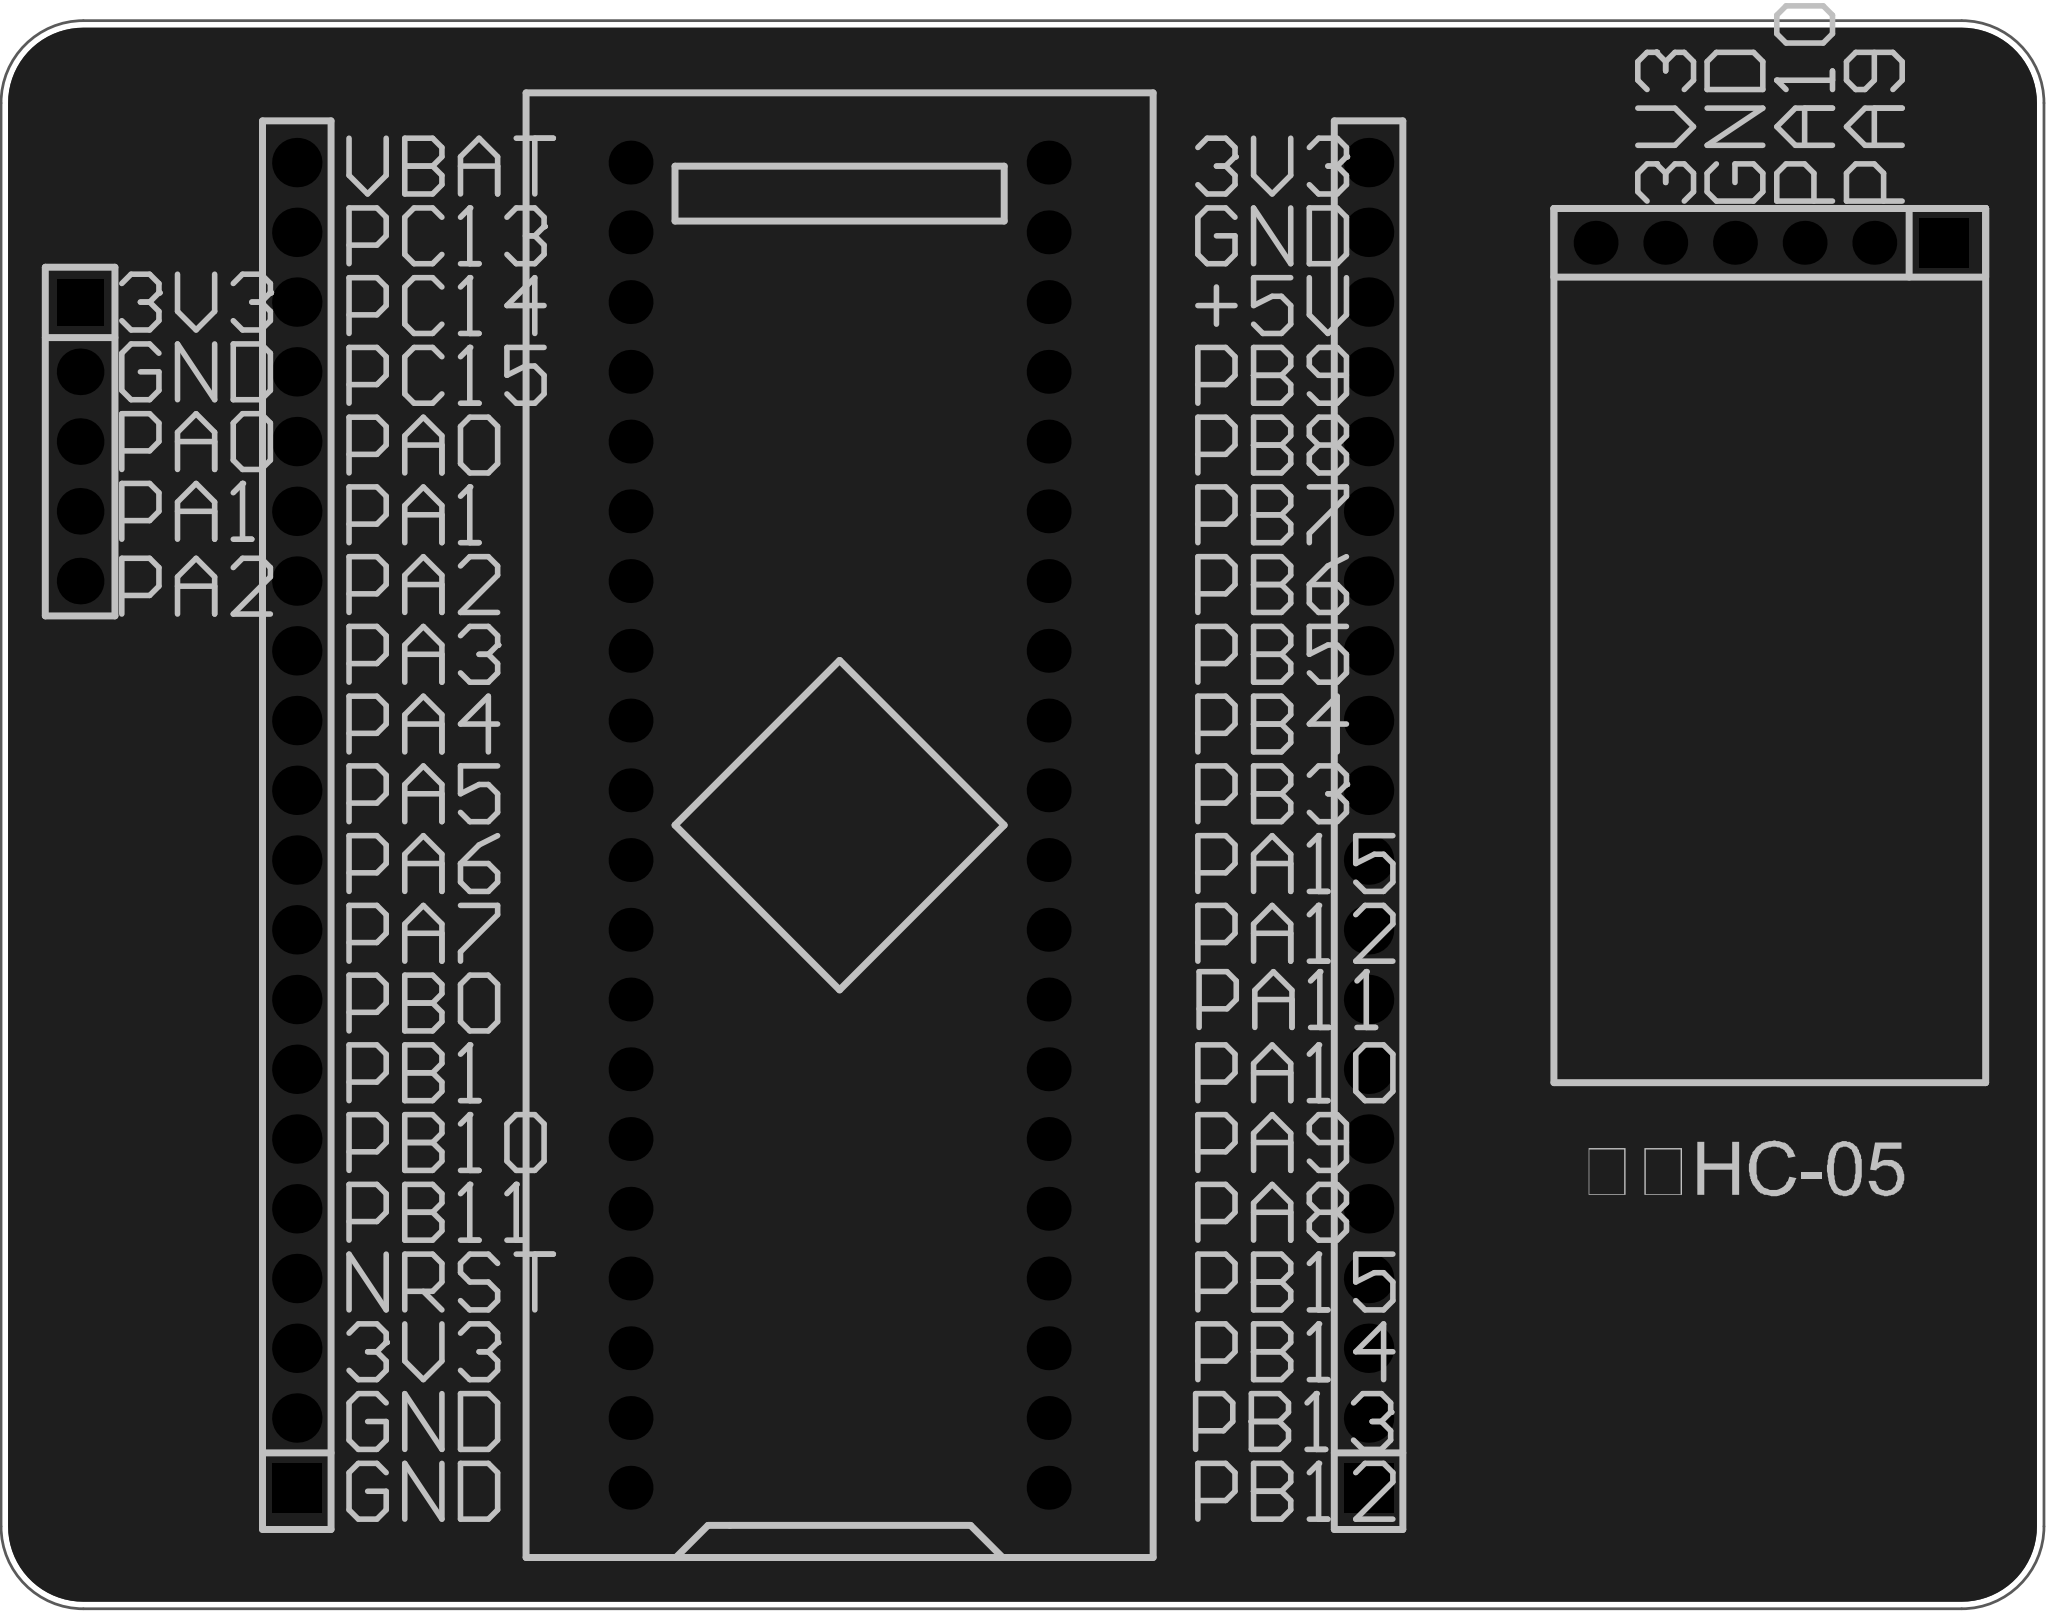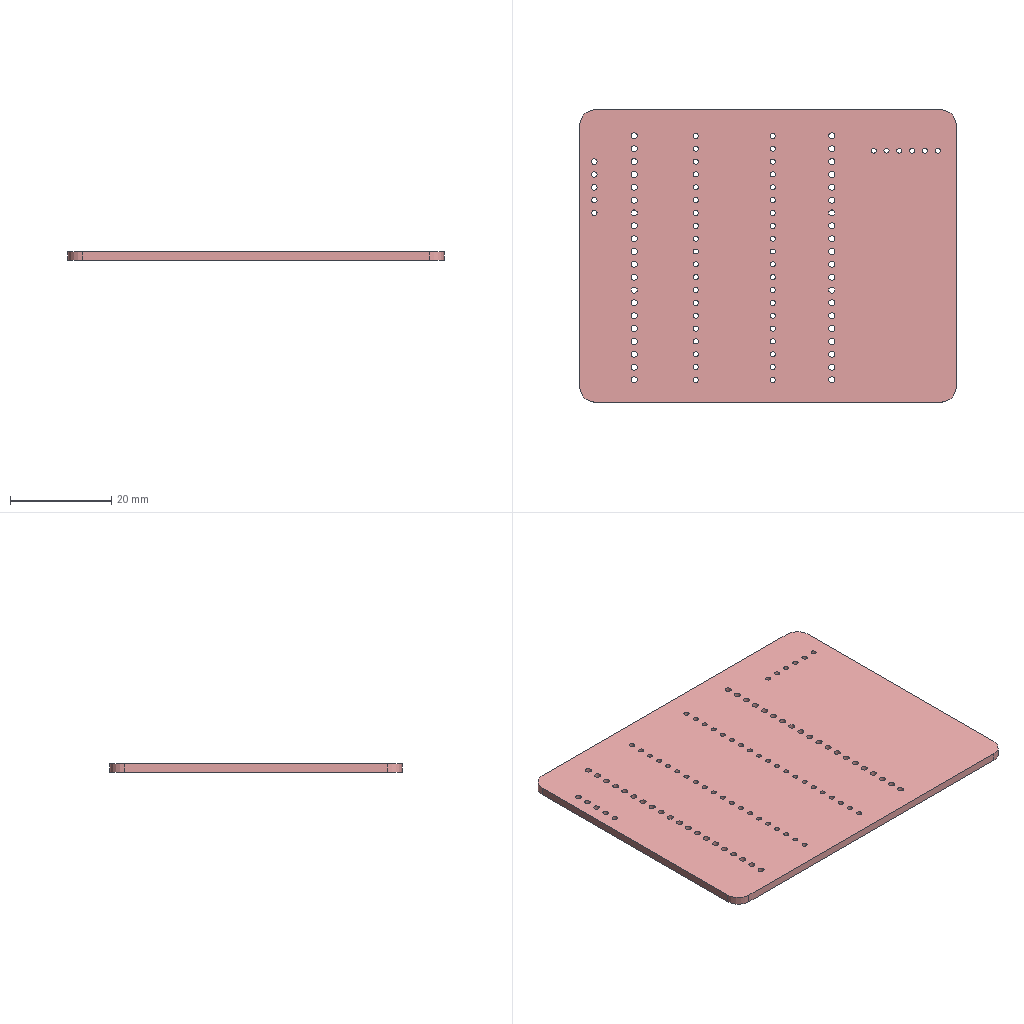Circuit board layout | Altium Designer | box 74.5 x 57.8 x 1.6 mm
Layer stack:
# Altium Designer layer stack of  (unit mm; dielectric type: 0 none, 1 core, 2 prepreg, 3 surface material)
index,name,kind,layer,copper_thickness_mm,dielectric_type,dielectric_thickness_mm,dielectric_material,dielectric_constant
0,Top Paste Mask Layer,other,,,,,,
1,Top Silkscreen Layer,other,,,,,,
2,Top Solder Mask Layer,dielectric,,,3,0.01,,3.3
3,Top Layer,copper,Top Layer,0.035,,,,
4,Dielectric1,dielectric,,,3,1.51,FR4,4.5
5,Bottom Layer,copper,Bottom Layer,0.035,,,,
6,Bottom Solder Mask Layer,dielectric,,,3,0.01,,3.3
7,Bottom Silkscreen Layer,other,,,,,,
8,Bottom Paste Mask Layer,other,,,,,,
# drill layer pairs: low layer,high layer
drill_pair,Top Layer,Bottom Layer
Part placement:
Designator,Comment,Layer,Footprint,Center-X(mm),Center-Y(mm),Rotation
U1,STM32F103C8T6-Card,TopLayer,CONN-TH_L53.3-W22.9_STM32F103C8T6-CARD,132.334,129.032,90
H1,,TopLayer,HDR-TH_20P-P2.54-V-F,151.617,129.032,90
H2,,TopLayer,HDR-TH_20P-P2.54-V-F,112.546,129.032,90
H4,,TopLayer,HDR-TH_6P-P2.54-V-F,166.243,150.241,180
H3,,TopLayer,HDR-TH_5P-P2.54-V-M,104.648,143.002,270
Pad and via stacks:
# Altium Designer via and pad stacks of  (unit mm). Each distinct definition once, with the count of objects using it.
# via: kind,start_layer,end_layer,hole_mm,diameter_mm,mode(0 simple;1 top-mid-bottom;2 full stack),diameter_per_layer,count,example_net
# pad: kind,layer,hole_mm,hole_type(0 round;1 square;2 slot),plating,top_size,top_shape(1 round;2 rect;3 octagon;9 rounded rect),mid_size,bottom_size,mode,footprint,size_per_layer,count,example
pad,Multi-Layer,1,0,plated,1.6x1.6,1,1.6x1.6,1.6x1.6,0,CONN-TH_L53.3-W22.9_STM32F103C8T6-CARD,,40,U1.1
pad,Multi-Layer,1.2,0,plated,1.8x1.8,2,1.8x1.8,1.8x1.8,0,HDR-TH_20P-P2.54-V-F,,2,H1.1
pad,Multi-Layer,1.2,0,plated,1.8x1.8,1,1.8x1.8,1.8x1.8,0,HDR-TH_20P-P2.54-V-F,,38,H1.2
pad,Multi-Layer,1.02,0,plated,1.6x1.6,1,1.6x1.6,1.6x1.6,0,HDR-TH_6P-P2.54-V-F,,5,H4.6
pad,Multi-Layer,1.02,0,plated,1.8x1.8,2,1.8x1.8,1.8x1.8,0,HDR-TH_6P-P2.54-V-F,,1,H4.1
pad,Multi-Layer,1.1,0,plated,1.7x1.7,2,1.7x1.7,1.7x1.7,0,HDR-TH_5P-P2.54-V-M,,1,H3.1
pad,Multi-Layer,1.1,0,plated,1.7x1.7,1,1.7x1.7,1.7x1.7,0,HDR-TH_5P-P2.54-V-M,,4,H3.2
Copper pours:
name,layer,net,type(0 solid;1 hatched;2 none)
Bottom Layer-GND,Bottom Layer,GND,0
Top Layer-GND,Top Layer,GND,0